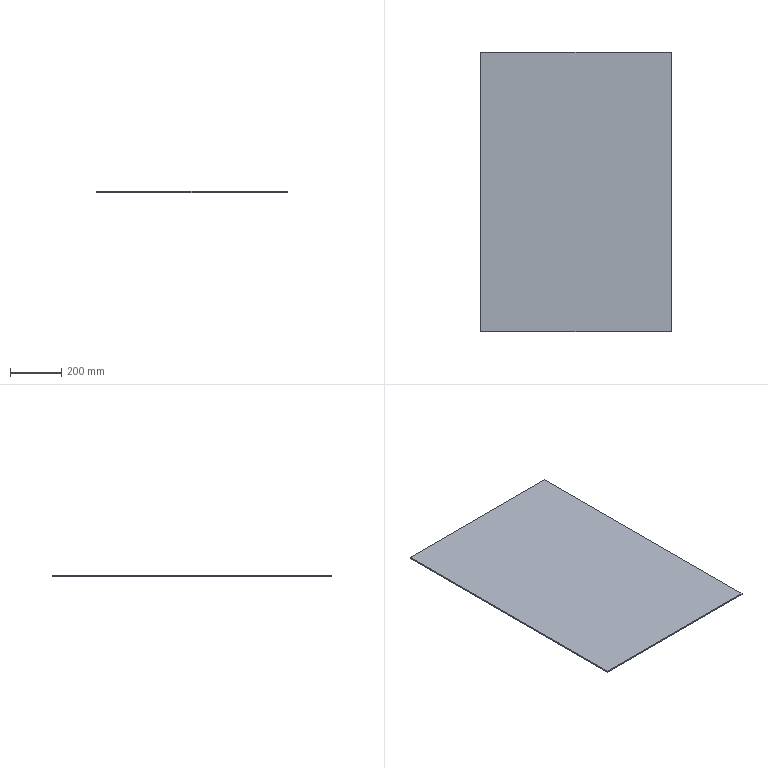Part | SolidWorks | features Extrusion 1, HoleWzd 1 | 1 solid | 6 faces | box 745 x 1091 x 5 mm | volume 4063975 mm3 | plane 6
STEP:
#1=CARTESIAN_POINT('',(372.5,-545.5,0.));
#2=VERTEX_POINT('',#1);
#3=CARTESIAN_POINT('',(372.5,545.5,0.));
#4=VERTEX_POINT('',#3);
#5=CARTESIAN_POINT('',(372.5,545.5,0.));
#6=DIRECTION('',(0.,1.,0.));
#7=VECTOR('',#6,1000.);
#8=LINE('',#5,#7);
#9=EDGE_CURVE('',#2,#4,#8,.T.);
#10=ORIENTED_EDGE('',*,*,#9,.T.);
#11=CARTESIAN_POINT('',(372.5,545.5,5.));
#12=VERTEX_POINT('',#11);
#13=CARTESIAN_POINT('',(372.5,545.5,5.));
#14=DIRECTION('',(0.,0.,-1.));
#15=VECTOR('',#14,1000.);
#16=LINE('',#13,#15);
#17=EDGE_CURVE('',#12,#4,#16,.T.);
#18=ORIENTED_EDGE('',*,*,#17,.F.);
#19=CARTESIAN_POINT('',(372.5,-545.5,5.));
#20=VERTEX_POINT('',#19);
#21=CARTESIAN_POINT('',(372.5,545.5,5.));
#22=DIRECTION('',(0.,1.,0.));
#23=VECTOR('',#22,1000.);
#24=LINE('',#21,#23);
#25=EDGE_CURVE('',#20,#12,#24,.T.);
#26=ORIENTED_EDGE('',*,*,#25,.F.);
#27=CARTESIAN_POINT('',(372.5,-545.5,5.));
#28=DIRECTION('',(0.,0.,-1.));
#29=VECTOR('',#28,1000.);
#30=LINE('',#27,#29);
#31=EDGE_CURVE('',#20,#2,#30,.T.);
#32=ORIENTED_EDGE('',*,*,#31,.T.);
#33=EDGE_LOOP('',(#10,#18,#26,#32));
#34=FACE_OUTER_BOUND('',#33,.T.);
#35=CARTESIAN_POINT('',(372.5,545.5,5.));
#36=DIRECTION('',(-1.,0.,0.));
#37=DIRECTION('',(0.,-1.,0.));
#38=AXIS2_PLACEMENT_3D('',#35,#36,#37);
#39=PLANE('',#38);
#40=ADVANCED_FACE('',(#34),#39,.F.);
#41=CARTESIAN_POINT('',(-372.5,545.5,0.));
#42=VERTEX_POINT('',#41);
#43=CARTESIAN_POINT('',(-372.5,545.5,0.));
#44=DIRECTION('',(-1.,0.,0.));
#45=VECTOR('',#44,1000.);
#46=LINE('',#43,#45);
#47=EDGE_CURVE('',#4,#42,#46,.T.);
#48=ORIENTED_EDGE('',*,*,#47,.T.);
#49=CARTESIAN_POINT('',(-372.5,545.5,5.));
#50=VERTEX_POINT('',#49);
#51=CARTESIAN_POINT('',(-372.5,545.5,5.));
#52=DIRECTION('',(0.,0.,-1.));
#53=VECTOR('',#52,1000.);
#54=LINE('',#51,#53);
#55=EDGE_CURVE('',#50,#42,#54,.T.);
#56=ORIENTED_EDGE('',*,*,#55,.F.);
#57=CARTESIAN_POINT('',(-372.5,545.5,5.));
#58=DIRECTION('',(-1.,0.,0.));
#59=VECTOR('',#58,1000.);
#60=LINE('',#57,#59);
#61=EDGE_CURVE('',#12,#50,#60,.T.);
#62=ORIENTED_EDGE('',*,*,#61,.F.);
#63=ORIENTED_EDGE('',*,*,#17,.T.);
#64=EDGE_LOOP('',(#48,#56,#62,#63));
#65=FACE_OUTER_BOUND('',#64,.T.);
#66=CARTESIAN_POINT('',(-372.5,545.5,5.));
#67=DIRECTION('',(0.,-1.,0.));
#68=DIRECTION('',(0.,0.,-1.));
#69=AXIS2_PLACEMENT_3D('',#66,#67,#68);
#70=PLANE('',#69);
#71=ADVANCED_FACE('',(#65),#70,.F.);
#72=CARTESIAN_POINT('',(-372.5,-545.5,0.));
#73=VERTEX_POINT('',#72);
#74=CARTESIAN_POINT('',(-372.5,545.5,0.));
#75=DIRECTION('',(0.,-1.,0.));
#76=VECTOR('',#75,1000.);
#77=LINE('',#74,#76);
#78=EDGE_CURVE('',#42,#73,#77,.T.);
#79=ORIENTED_EDGE('',*,*,#78,.T.);
#80=CARTESIAN_POINT('',(-372.5,-545.5,5.));
#81=VERTEX_POINT('',#80);
#82=CARTESIAN_POINT('',(-372.5,-545.5,5.));
#83=DIRECTION('',(0.,0.,-1.));
#84=VECTOR('',#83,1000.);
#85=LINE('',#82,#84);
#86=EDGE_CURVE('',#81,#73,#85,.T.);
#87=ORIENTED_EDGE('',*,*,#86,.F.);
#88=CARTESIAN_POINT('',(-372.5,545.5,5.));
#89=DIRECTION('',(0.,-1.,0.));
#90=VECTOR('',#89,1000.);
#91=LINE('',#88,#90);
#92=EDGE_CURVE('',#50,#81,#91,.T.);
#93=ORIENTED_EDGE('',*,*,#92,.F.);
#94=ORIENTED_EDGE('',*,*,#55,.T.);
#95=EDGE_LOOP('',(#79,#87,#93,#94));
#96=FACE_OUTER_BOUND('',#95,.T.);
#97=CARTESIAN_POINT('',(-372.5,545.5,5.));
#98=DIRECTION('',(1.,0.,0.));
#99=DIRECTION('',(0.,1.,0.));
#100=AXIS2_PLACEMENT_3D('',#97,#98,#99);
#101=PLANE('',#100);
#102=ADVANCED_FACE('',(#96),#101,.F.);
#103=CARTESIAN_POINT('',(-372.5,-545.5,0.));
#104=DIRECTION('',(1.,0.,0.));
#105=VECTOR('',#104,1000.);
#106=LINE('',#103,#105);
#107=EDGE_CURVE('',#73,#2,#106,.T.);
#108=ORIENTED_EDGE('',*,*,#107,.T.);
#109=ORIENTED_EDGE('',*,*,#31,.F.);
#110=CARTESIAN_POINT('',(-372.5,-545.5,5.));
#111=DIRECTION('',(1.,0.,0.));
#112=VECTOR('',#111,1000.);
#113=LINE('',#110,#112);
#114=EDGE_CURVE('',#81,#20,#113,.T.);
#115=ORIENTED_EDGE('',*,*,#114,.F.);
#116=ORIENTED_EDGE('',*,*,#86,.T.);
#117=EDGE_LOOP('',(#108,#109,#115,#116));
#118=FACE_OUTER_BOUND('',#117,.T.);
#119=CARTESIAN_POINT('',(-372.5,-545.5,5.));
#120=DIRECTION('',(0.,1.,0.));
#121=DIRECTION('',(0.,0.,1.));
#122=AXIS2_PLACEMENT_3D('',#119,#120,#121);
#123=PLANE('',#122);
#124=ADVANCED_FACE('',(#118),#123,.F.);
#125=ORIENTED_EDGE('',*,*,#25,.T.);
#126=ORIENTED_EDGE('',*,*,#61,.T.);
#127=ORIENTED_EDGE('',*,*,#92,.T.);
#128=ORIENTED_EDGE('',*,*,#114,.T.);
#129=EDGE_LOOP('',(#125,#126,#127,#128));
#130=FACE_OUTER_BOUND('',#129,.T.);
#131=CARTESIAN_POINT('',(0.,0.,5.));
#132=DIRECTION('',(0.,0.,1.));
#133=DIRECTION('',(1.,0.,0.));
#134=AXIS2_PLACEMENT_3D('',#131,#132,#133);
#135=PLANE('',#134);
#136=ADVANCED_FACE('',(#130),#135,.T.);
#137=ORIENTED_EDGE('',*,*,#9,.F.);
#138=ORIENTED_EDGE('',*,*,#107,.F.);
#139=ORIENTED_EDGE('',*,*,#78,.F.);
#140=ORIENTED_EDGE('',*,*,#47,.F.);
#141=EDGE_LOOP('',(#137,#138,#139,#140));
#142=FACE_OUTER_BOUND('',#141,.T.);
#143=CARTESIAN_POINT('',(0.,0.,0.));
#144=DIRECTION('',(0.,0.,1.));
#145=DIRECTION('',(1.,0.,0.));
#146=AXIS2_PLACEMENT_3D('',#143,#144,#145);
#147=PLANE('',#146);
#148=ADVANCED_FACE('',(#142),#147,.F.);
#149=CLOSED_SHELL('',(#40,#71,#102,#124,#136,#148));
#150=MANIFOLD_SOLID_BREP('',#149);
#151=CARTESIAN_POINT('',(0.,0.,0.));
#152=DIRECTION('',(0.,0.,1.));
#153=DIRECTION('',(1.,0.,0.));
#154=AXIS2_PLACEMENT_3D('',#151,#152,#153);
#155=(LENGTH_UNIT()NAMED_UNIT(*)SI_UNIT(.MILLI.,.METRE.));
#156=UNCERTAINTY_MEASURE_WITH_UNIT(LENGTH_MEASURE(0.00001),#155,'','');
#157=(NAMED_UNIT(*)PLANE_ANGLE_UNIT()SI_UNIT($,.RADIAN.));
#158=(NAMED_UNIT(*)SI_UNIT($,.STERADIAN.)SOLID_ANGLE_UNIT());
#159=(GEOMETRIC_REPRESENTATION_CONTEXT(3)GLOBAL_UNCERTAINTY_ASSIGNED_CONTEXT((#156))GLOBAL_UNIT_ASSIGNED_CONTEXT((#155,#157,#158))REPRESENTATION_CONTEXT('',''));
#160=ADVANCED_BREP_SHAPE_REPRESENTATION('',(#150,#154),#159);